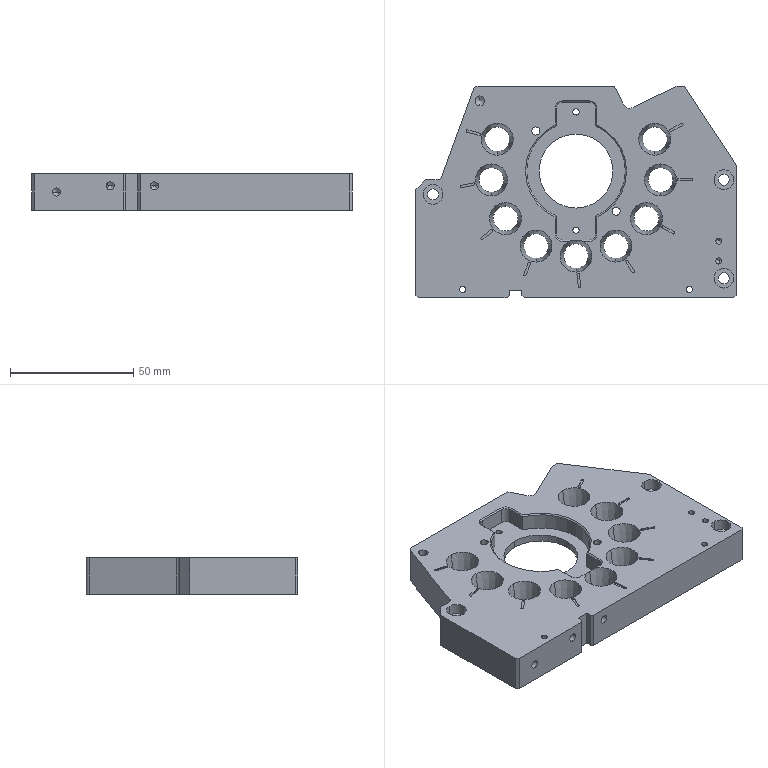NC program | NX | posted with a generic post | part box 130 x 86 x 15 mm
Lines 1 to 920 of 5031:
N10 G17 G21 G94 G90
(ADAPTIVE_MILLING_COPY , TOOL : D10)
N12 T04 M6
N14 G54
N16 G17 G0 G90 X11.01 Y-3.735 B0. C0. S7500 M3
N18 G43 Z30. H4
N20 Z3.
N22 G94 G3 X11.01 Y-3.735 Z2.506 I-2.51 J3.735 F1000.
N24 X11.01 Y-3.735 Z2.013 I-2.51 J3.735
N26 X11.01 Y-3.735 Z1.519 I-2.51 J3.735
N28 X11.01 Y-3.735 Z1.026 I-2.51 J3.735
N30 X11.01 Y-3.735 Z0.532 I-2.51 J3.735
N32 X11.01 Y-3.735 Z0.039 I-2.51 J3.735
N34 X11.01 Y-3.735 Z-0.455 I-2.51 J3.735
N36 X11.01 Y-3.735 Z-0.948 I-2.51 J3.735
N38 X11.01 Y-3.735 Z-1.442 I-2.51 J3.735
N40 X11.01 Y-3.735 Z-1.935 I-2.51 J3.735
N42 X11.01 Y-3.735 Z-2.429 I-2.51 J3.735
N44 X11.01 Y-3.735 Z-2.922 I-2.51 J3.735
N46 X11.01 Y-3.735 Z-3.416 I-2.51 J3.735
N48 X11.01 Y-3.735 Z-3.909 I-2.51 J3.735
N50 X11.01 Y-3.735 Z-4.403 I-2.51 J3.735
N52 X8.5 Y-4.5 Z-4.85 R-4.5
N54 X7.534 Y-4.399 R-4.499 F3000.
N56 X7.216 Y4.39 R-4.547
N58 X13.113 Y0.575 R-4.602
N60 X8.819 Y-4.663 R-4.652
N62 X4.804 Y2.943 R-4.71
N64 X10.9 Y4.161 R-4.762
N66 X10.384 Y-4.465 R-4.814
N68 X3.834 Y-1.432 R-4.875
N70 X7.652 Y4.886 R-4.926
N72 X13.531 Y-0.204 R-4.986
N74 X8.679 Y-5.061 R-5.039
N76 X4.13 Y2.665 R-5.102
N78 X10.535 Y4.785 R-5.156
N80 X11.506 Y-4.309 R-5.215
N82 X4.9 Y-3.869 R-5.277
N84 X6.445 Y4.953 R-5.333
N86 X13.444 Y2.278 R-5.398
N88 X9.278 Y-5.426 R-5.452
N90 X3.211 Y1.618 R-5.516
N92 X9.379 Y5.545 R-5.571
N94 X12.858 Y-3.644 R-5.637
N96 X5.804 Y-5.037 R-5.698
N98 X5.483 Y4.937 R-5.759
N100 X13.196 Y3.521 R-5.825
N102 X9.953 Y-5.735 R-5.882
N104 X2.549 Y0.352 R-5.949
N106 X9.096 Y6.019 R-6.007
N108 X13.682 Y-3.259 R-6.074
N110 X5.984 Y-5.618 R-6.137
N112 X5.083 Y5.205 R-6.201
N114 X13.852 Y3.35 R-6.267
N116 X9.625 Y-6.261 R-6.327
N118 X2.135 Y0.757 R-6.396
N120 X9.87 Y6.355 R-6.457
N122 X13.697 Y-4.024 R-6.526
N124 X4.883 Y-5.533 R-6.591
N126 X5.308 Y5.875 R-6.658
N128 X14.682 Y2.776 R-6.726
N130 X9.232 Y-6.786 R-6.79
N132 X1.734 Y1.224 R-6.86
N134 X10.363 Y6.717 R-6.925
N136 X14.11 Y-4.259 R-6.996
N138 X4.048 Y-5.51 R-7.064
N140 X5.623 Y6.56 R-7.132
N142 X15.557 Y1.686 R-7.203
N144 X8.369 Y-7.302 R-7.269
N146 X1.72 Y2.864 R-7.341
N148 X11.996 Y6.587 R-7.409
N150 X13.441 Y-5.676 R-7.48
N152 X2.184 Y-4.172 R-7.552
N154 X6.418 Y7.367 R-7.621
N156 X16.249 Y0.004 R-7.694
N158 X6.999 Y-7.65 R-7.764
N160 X1.855 Y4.197 R-7.838
N162 X13.622 Y6.092 R-7.909
N164 X12.463 Y-6.977 R-7.981
N166 X0.759 Y-2.294 R-8.055
N168 X8.58 Y8.165 R-8.126
N170 X16.024 Y-3.391 R-8.2
N172 X4.076 Y-7.019 R-8.271
N174 X3.755 Y6.902 R-8.346
N176 X16.386 Y3.104 R-8.42
N178 X9.181 Y-8.502 R-8.493
N180 X0.384 Y2.814 R-8.568
N182 X12.846 Y7.523 R-8.641
N184 X13.786 Y-6.989 R-8.716
N186 X0.145 Y-2.797 R-8.791
N188 X8.261 Y8.9 R-8.865
N190 X16.689 Y-3.723 R-8.94
N192 X2.926 Y-7.118 R-9.016
N194 X3.694 Y7.755 R-9.091
N196 X17.471 Y2.139 R-9.168
N198 X7.96 Y-9.265 R-9.244
N200 X-0.042 Y3.787 R-9.32
N202 X14.255 Y7.492 R-9.399
N204 X14. Y-7.775 R-9.475
N206 X-0.954 Y-1.506 R-9.553
N208 X10.23 Y9.516 R-9.629
N210 X16.905 Y-4.958 R-9.706
N212 X0.52 Y-5.707 R-9.784
N214 X5.806 Y9.521 R-9.861
N216 X18.258 Y-2.168 R-9.939
N218 X3.239 Y-8.561 R-10.016
N220 X2.227 Y7.946 R-10.094
N222 X18.392 Y2.605 R-10.173
N224 X8.118 Y-10.287 R-10.253
N226 X-0.877 Y4.4 R-10.332
N228 X15.771 Y7.521 R-10.413
N230 X13.155 Y-9.458 R-10.492
N232 X-2.06 Y0.845 R-10.571
N234 X12.822 Y9.783 R-10.651
N236 X16.267 Y-7.48 R-10.73
N238 X-1.831 Y-3.275 R-10.812
N240 X8.884 Y10.921 R-10.89
N242 X18.073 Y-5.475 R-10.971
N244 X-0.415 Y-6.584 R-11.051
N246 X4.875 Y10.558 R-11.132
N248 X19.445 Y-2.701 R-11.213
N250 X2.721 Y-9.748 R-11.295
N252 X1.679 Y9.143 R-11.376
N254 X19.807 Y2.176 R-11.46
N256 X7.244 Y-11.519 R-11.542
N258 X-0.899 Y6.883 R-11.623
N260 X18.674 Y5.893 R-11.706
N262 X11.097 Y-11.55 R-11.788
N264 X-2.517 Y4.491 R-11.871
N266 X16.44 Y8.998 R-11.954
N268 X13.838 Y-10.849 R-12.037
N270 X-3.507 Y1.841 R-12.119
N272 X14.292 Y10.787 R-12.202
N274 X15.907 Y-9.872 R-12.284
N276 X-3.821 Y-1.403 R-12.369
N278 X10.875 Y12.262 R-12.452
N280 X18.058 Y-8.202 R-12.537
N282 X-2.904 Y-5.494 R-12.622
N284 X7.733 Y12.715 R-12.705
N286 X19.26 Y-7.025 R-12.79
N288 X-1.417 Y-8.272 R-12.875
N290 X4.621 Y12.399 R-12.959
N292 X20.867 Y-4.326 R-13.045
N294 X0.656 Y-10.584 R-13.13
N296 X2.615 Y11.865 R-13.214
N298 X21.723 Y-1.882 R-13.301
N300 X2.704 Y-12.118 R-13.385
N302 X1.622 Y11.617 R-13.471
N304 X22.108 Y0.122 R-13.556
N306 X3.966 Y-12.919 R-13.642
N308 X1.115 Y11.607 R-13.727
N310 X22.2 Y2.124 R-13.814
N312 X5.792 Y-13.687 R-13.899
N314 X-0.216 Y10.974 R-13.986
N316 X22.159 Y3.581 R-14.072
N318 X6.615 Y-14.086 R-14.158
N320 X-0.665 Y10.944 R-14.244
N322 X22.156 Y4.493 R-14.331
N324 X6.903 Y-14.384 R-14.417
N326 X-0.683 Y11.265 R-14.504
N328 X22.47 Y4.368 R-14.59
N330 X6.639 Y-14.614 R-14.677
N332 X-0.687 Y11.599 R-14.764
N334 X22.784 Y4.222 R-14.852
N336 X5.817 Y-14.752 R-14.938
N338 X-0.232 Y12.265 R-15.026
N340 X23.361 Y2.993 R-15.113
N342 X4.981 Y-14.844 R-15.2
N344 X0.258 Y12.915 R-15.288
N346 X23.754 Y2.261 R-15.377
N348 X4.137 Y-14.894 R-15.463
N350 X1.273 Y13.806 R-15.552
N352 X24.158 Y0.954 R-15.64
N354 X2.766 Y-14.705 R-15.728
N356 X2.355 Y14.609 R-15.816
N358 X24.447 Y-0.379 R-15.905
N360 X1.423 Y-14.406 R-15.993
N362 X3.492 Y15.316 R-16.083
N364 X24.557 Y-2.283 R-16.171
N366 X0.121 Y-14. R-16.26
N368 X23.587 Y-6.301 R16.319
N370 X7.298 Y16.333 R16.374
N372 X-7.85 Y1.664 R16.374
N374 X-7.715 Y-2.654 R30.055
N376 X6.448 Y-16.35 R16.43
N378 X11.019 Y-16.271 R45.472
N380 X24.849 Y-2.38 R16.457
N382 G1 X24.85 Y0.425
N384 G3 X22.67 Y8.512 R14.212
N386 X10.995 Y16.35 R16.548
N388 X9.932 Y15.532 R1.108
N390 X10.262 Y14.424 Z-4.789 R1.127
N392 G1 X10.8 Y13.853 Z-4.75
N394 X22.33 Y1.627
N396 X22.7 Y1.23 Z-4.777
N398 X23.086 Y0.848 Z-4.804
N400 G3 X23.95 Y0.643 Z-4.85 R1.127
N402 X24.85 Y1.725 R1.106
N404 X23.606 Y7.078 R11.456
N406 X11.828 Y16.35 R16.66
N408 X10.766 Y15.535 R1.108
N410 X11.093 Y14.426 Z-4.789 R1.127
N412 G1 X11.63 Y13.853 Z-4.75
N414 X22.33 Y2.431
N416 X22.699 Y2.033 Z-4.777
N418 X23.083 Y1.65 Z-4.804
N420 G3 X23.947 Y1.442 Z-4.85 R1.127
N422 X24.85 Y2.525 R1.106
N424 X23.791 Y7.034 R9.912
N426 X12.504 Y16.349 R16.748
N428 X11.442 Y15.538 R1.108
N430 X11.765 Y14.428 Z-4.789 R1.127
N432 G1 X12.299 Y13.853 Z-4.75
N434 X22.331 Y3.061
N436 X23.059 Y2.294 Z-4.803
N438 G3 X23.943 Y2.067 Z-4.85 R1.118
N440 X24.85 Y3.15 R1.106
N442 X23.859 Y7.241 R8.92
N444 X13.073 Y16.349 R16.704
N446 X12.012 Y15.54 R1.108
N448 X12.332 Y14.43 Z-4.789 R1.127
N450 G1 X12.865 Y13.853 Z-4.75
N452 X22.331 Y3.615
N454 X23.057 Y2.846 Z-4.803
N456 G3 X23.941 Y2.616 Z-4.85 R1.118
N458 X24.85 Y3.7 R1.106
N460 X23.858 Y7.585 R8.289
N462 X13.612 Y16.345 R16.68
N464 G1 X13.587 Y16.348
N466 X13.562 Y16.35
N468 G3 X12.501 Y15.541 R1.108
N470 X12.82 Y14.432 Z-4.789 R1.127
N472 G1 X13.353 Y13.853 Z-4.75
N474 X22.331 Y4.116
N476 X23.056 Y3.347 Z-4.803
N478 G3 X23.94 Y3.116 Z-4.85 R1.118
N480 X24.85 Y4.2 R1.106
N482 X23.949 Y7.725 R7.576
N484 X14.121 Y16.339 R16.718
N486 G1 X14.096 Y16.342
N488 X14.071 Y16.345
N490 X14.046 Y16.348
N492 X14.021 Y16.35
N494 G3 X12.961 Y15.543 R1.108
N496 X13.277 Y14.433 Z-4.789 R1.127
N498 G1 X13.81 Y13.853 Z-4.75
N500 X22.331 Y4.569
N502 X23.054 Y3.798 Z-4.803
N504 G3 X23.938 Y3.566 Z-4.85 R1.117
N506 X24.85 Y4.65 R1.106
N508 X23.928 Y8.091 R7.237
N510 X14.575 Y16.334 R16.618
N512 G1 X14.551 Y16.338
N514 X14.526 Y16.342
N516 X14.501 Y16.345
N518 X14.476 Y16.347
N520 X14.451 Y16.349
N522 G3 X13.392 Y15.546 R1.108
N524 X13.705 Y14.435 Z-4.789 R1.127
N526 G1 X14.236 Y13.853 Z-4.75
N528 X22.331 Y4.974
N530 X23.051 Y4.2 Z-4.803
N532 G3 X23.934 Y3.965 Z-4.85 R1.117
N534 X24.85 Y5.05 R1.106
N536 X23.9 Y8.455 R6.966
N538 X15.025 Y16.323 R16.604
N540 G1 X15.001 Y16.328
N542 X14.976 Y16.333
N544 X14.952 Y16.338
N546 X14.927 Y16.341
N548 X14.902 Y16.344
N550 X14.877 Y16.347
N552 X14.853 Y16.349
N554 G3 X13.794 Y15.547 R1.108
N556 X14.104 Y14.437 Z-4.789 R1.127
N558 G1 X14.634 Y13.853 Z-4.75
N560 X22.331 Y5.376
N562 X23.049 Y4.602 Z-4.803
N564 G3 X23.932 Y4.365 Z-4.85 R1.117
N566 X24.85 Y5.45 R1.106
N568 X23.97 Y8.618 R6.515
N570 X15.447 Y16.312 R16.495
N572 G1 X15.422 Y16.318
N574 X15.398 Y16.324
N576 X15.374 Y16.33
N578 X15.349 Y16.334
N580 X15.325 Y16.338
N582 X15.3 Y16.342
N584 X15.275 Y16.345
N586 X15.25 Y16.348
N588 X15.225 Y16.349
N590 G3 X14.167 Y15.549 R1.108
N592 X14.476 Y14.438 Z-4.79 R1.127
N594 G1 X15.005 Y13.853 Z-4.75
N596 X22.331 Y5.754
N598 X23.048 Y4.978 Z-4.803
N600 G3 X23.931 Y4.74 Z-4.85 R1.117
N602 X24.85 Y5.825 R1.106
N604 X23.957 Y8.937 R6.318
N606 X15.839 Y16.302 R16.322
N608 G1 X15.816 Y16.309
N610 X15.791 Y16.316
N612 X15.767 Y16.322
N614 X15.743 Y16.328
N616 X15.718 Y16.333
N618 X15.694 Y16.337
N620 X15.669 Y16.341
N622 X15.644 Y16.344
N624 X15.619 Y16.347
N626 X15.594 Y16.349
N628 G3 X14.537 Y15.551 R1.108
N630 X14.842 Y14.44 Z-4.79 R1.127
N632 G1 X15.37 Y13.853 Z-4.75
N634 X22.331 Y6.108
N636 X23.045 Y5.33 Z-4.803
N638 G3 X23.928 Y5.089 Z-4.85 R1.117
N640 X24.85 Y6.175 R1.106
N642 X23.952 Y9.233 R6.12
N644 X16.276 Y16.272 R16.312
N646 G1 X16.205 Y16.296
N648 X16.157 Y16.311
N650 X16.133 Y16.317
N652 X16.108 Y16.323
N654 X16.084 Y16.329
N656 X16.059 Y16.334
N658 X16.035 Y16.338
N660 X16.01 Y16.342
N662 X15.985 Y16.345
N664 X15.96 Y16.347
N666 X15.935 Y16.349
N668 G3 X14.878 Y15.554 R1.108
N670 X15.181 Y14.443 Z-4.79 R1.127
N672 G1 X15.708 Y13.853 Z-4.75
N674 X22.331 Y6.437
N676 X23.042 Y5.658 Z-4.803
N678 G3 X23.925 Y5.414 Z-4.85 R1.117
N680 X24.85 Y6.5 R1.106
N682 X23.978 Y9.462 R5.87
N684 X16.661 Y16.253 R16.132
N686 G1 X16.59 Y16.278
N688 X16.519 Y16.302
N690 X16.495 Y16.309
N692 X16.471 Y16.316
N694 X16.447 Y16.322
N696 X16.422 Y16.328
N698 X16.398 Y16.333
N700 X16.373 Y16.337
N702 X16.348 Y16.341
N704 X16.324 Y16.344
N706 X16.299 Y16.347
N708 X16.274 Y16.349
N710 G3 X15.218 Y15.556 R1.108
N712 X15.517 Y14.445 Z-4.79 R1.127
N714 G1 X16.042 Y13.853 Z-4.75
N716 X22.331 Y6.766
N718 X23.04 Y5.985 Z-4.803
N720 G3 X23.922 Y5.738 Z-4.85 R1.117
N722 X24.85 Y6.825 R1.106
N724 X23.979 Y9.734 R5.708
N726 X16.995 Y16.248 R15.815
N728 G1 X16.925 Y16.273
N730 X16.854 Y16.298
N732 X16.83 Y16.305
N734 X16.806 Y16.312
N736 X16.782 Y16.319
N738 X16.757 Y16.325
N740 X16.733 Y16.33
N742 X16.708 Y16.335
N744 X16.684 Y16.339
N746 X16.659 Y16.342
N748 X16.634 Y16.345
N750 X16.609 Y16.348
N752 X16.584 Y16.35
N754 G3 X15.528 Y15.557 R1.108
N756 X15.826 Y14.447 Z-4.79 R1.127
N758 G1 X16.351 Y13.853 Z-4.75
N760 X22.331 Y7.093
N762 X23.039 Y6.311 Z-4.803
N764 G3 X23.92 Y6.063 Z-4.85 R1.117
N766 X24.85 Y7.15 R1.106
N768 X23.94 Y10.072 R5.658
N770 X17.349 Y16.23 R15.574
N772 G1 X17.28 Y16.257
N774 X17.209 Y16.283
N776 X17.162 Y16.299
N778 X17.138 Y16.306
N780 X17.114 Y16.313
N782 X17.09 Y16.319
N784 X17.065 Y16.325
N786 X17.041 Y16.33
N788 X17.016 Y16.335
N790 X16.992 Y16.339
N792 X16.967 Y16.343
N794 X16.942 Y16.346
N796 X16.917 Y16.348
N798 X16.892 Y16.35
N800 G3 X15.837 Y15.559 R1.108
N802 X16.132 Y14.449 Z-4.79 R1.128
N804 G1 X16.656 Y13.853 Z-4.75
N806 X22.331 Y7.398
N808 X23.036 Y6.613 Z-4.803
N810 G3 X23.917 Y6.363 Z-4.85 R1.117
N812 X24.85 Y7.45 R1.106
N814 X23.934 Y10.343 R5.537
N816 X17.677 Y16.219 R15.23
N818 G1 X17.608 Y16.247
N820 X17.538 Y16.273
N822 X17.467 Y16.298
N824 X17.443 Y16.305
N826 X17.419 Y16.312
N828 X17.395 Y16.319
N830 X17.37 Y16.325
N832 X17.346 Y16.33
N834 X17.321 Y16.335
N836 X17.297 Y16.339
N838 X17.272 Y16.342
N840 X17.247 Y16.345
N842 X17.222 Y16.348
N844 X17.197 Y16.35
N846 G3 X16.143 Y15.562 R1.108
N848 X16.434 Y14.451 Z-4.79 R1.128
N850 G1 X16.957 Y13.853 Z-4.75
N852 X22.331 Y7.702
N854 X23.033 Y6.915 Z-4.803
N856 G3 X23.914 Y6.662 Z-4.85 R1.117
N858 X24.85 Y7.75 R1.106
N860 X23.951 Y10.571 R5.394
N862 X17.933 Y16.234 R14.657
N864 G1 X17.863 Y16.261
N866 X17.793 Y16.287
N868 X17.745 Y16.303
N870 X17.721 Y16.31
N872 X17.697 Y16.317
N874 X17.673 Y16.323
N876 X17.648 Y16.328
N878 X17.624 Y16.333
N880 X17.599 Y16.337
N882 X17.575 Y16.341
N884 X17.55 Y16.344
N886 X17.525 Y16.347
N888 X17.5 Y16.349
N890 G3 X16.446 Y15.565 R1.108
N892 X16.733 Y14.454 Z-4.79 R1.128
N894 G1 X17.253 Y13.853 Z-4.75
N896 X22.331 Y7.983
N898 X23.029 Y7.194 Z-4.803
N900 G3 X23.909 Y6.936 Z-4.85 R1.117
N902 X24.85 Y8.025 R1.106
N904 X23.94 Y10.841 R5.294
N906 X18.255 Y16.218 R14.31
N908 G1 X18.186 Y16.247
N910 X18.116 Y16.274
N912 X18.069 Y16.29
N914 X18.045 Y16.298
N916 X18.021 Y16.306
N918 X17.997 Y16.313
N920 X17.973 Y16.319
N922 X17.949 Y16.325
N924 X17.924 Y16.33
N926 X17.9 Y16.335
N928 X17.875 Y16.339
N930 X17.85 Y16.343
N932 X17.825 Y16.346
N934 X17.801 Y16.348
N936 X17.776 Y16.35
N938 G3 X16.722 Y15.566 R1.108
N940 X17.008 Y14.456 Z-4.79 R1.128
N942 G1 X17.528 Y13.853 Z-4.75
N944 X22.331 Y8.285
N946 X23.028 Y7.495 Z-4.803
N948 G3 X23.908 Y7.236 Z-4.85 R1.117
N950 X24.85 Y8.325 R1.106
N952 X23.966 Y11.046 R5.156
N954 X18.552 Y16.21 R13.864
N956 G1 X18.049 Y16.35
N958 G3 X16.996 Y15.568 R1.108
N960 X17.279 Y14.458 Z-4.79 R1.128
N962 G1 X17.798 Y13.853 Z-4.75
N964 X22.332 Y8.564
N966 X23.026 Y7.772 Z-4.803
N968 G3 X23.905 Y7.511 Z-4.85 R1.117
N970 X24.85 Y8.6 R1.106
N972 X23.912 Y11.38 R5.187
N974 X18.845 Y16.201 R13.419
N976 G1 X18.777 Y16.23
N978 X18.707 Y16.259
N980 X18.637 Y16.285
N982 X18.589 Y16.301
N984 X18.566 Y16.308
N986 X18.542 Y16.315
N988 X18.517 Y16.321
N990 X18.493 Y16.327
N992 X18.468 Y16.332
N994 X18.444 Y16.336
N996 X18.419 Y16.34
N998 X18.394 Y16.344
N1000 X18.37 Y16.346
N1002 X18.345 Y16.349
N1004 G3 X17.294 Y15.574 R1.108
N1006 X17.569 Y14.463 Z-4.79 R1.128
N1008 G1 X18.084 Y13.853 Z-4.75
N1010 X22.332 Y8.824
N1012 X23.02 Y8.027 Z-4.803
N1014 G3 X23.898 Y7.76 Z-4.85 R1.117
N1016 X24.85 Y8.85 R1.106
N1018 X23.986 Y11.498 R4.938
N1020 X19.091 Y16.209 R12.81
N1022 G1 X19.022 Y16.239
N1024 X18.975 Y16.258
N1026 X18.905 Y16.284
N1028 X18.858 Y16.3
N1030 X18.834 Y16.308
N1032 X18.81 Y16.315
N1034 X18.786 Y16.321
N1036 X18.762 Y16.327
N1038 X18.737 Y16.332
N1040 X18.713 Y16.336
N1042 X18.688 Y16.34
N1044 X18.663 Y16.343
N1046 X18.638 Y16.346
N1048 X18.613 Y16.348
N1050 G3 X17.563 Y15.577 R1.108
N1052 X17.835 Y14.465 Z-4.79 R1.128
N1054 G1 X18.348 Y13.853 Z-4.75
N1056 X22.332 Y9.104
N1058 X23.017 Y8.305 Z-4.803
N1060 G3 X23.894 Y8.034 Z-4.85 R1.117
N1062 X24.85 Y9.125 R1.106
N1064 X23.929 Y11.831 R4.984
N1066 X19.356 Y16.206 R12.272
N1068 G1 X18.855 Y16.35
N1070 G3 X17.805 Y15.579 R1.108
N1072 X18.125 Y14.407 Z-4.786 R1.183
N1074 G1 X18.587 Y13.853 Z-4.75
N1076 X22.332 Y9.358
N1078 X23.014 Y8.557 Z-4.803
N1080 G3 X23.891 Y8.284 Z-4.85 R1.117
N1082 X24.85 Y9.375 R1.106
N1084 X23.922 Y12.078 R4.925
N1086 X19.574 Y16.222 R11.593
N1088 G1 X19.528 Y16.242
N1090 X19.458 Y16.27
N1092 X19.411 Y16.287
N1094 X19.388 Y16.295
N1096 X19.364 Y16.303
N1098 X19.34 Y16.31
N1100 X19.316 Y16.317
N1102 X19.292 Y16.323
N1104 X19.267 Y16.328
N1106 X19.243 Y16.333
N1108 X19.218 Y16.338
N1110 X19.194 Y16.341
N1112 X19.169 Y16.344
N1114 X19.144 Y16.347
N1116 X19.119 Y16.349
N1118 G3 X18.071 Y15.583 R1.108
N1120 X18.385 Y14.41 Z-4.786 R1.183
N1122 G1 X18.844 Y13.853 Z-4.75
N1124 X22.332 Y9.616
N1126 X23.01 Y8.811 Z-4.803
N1128 G3 X23.885 Y8.533 Z-4.85 R1.117
N1130 X24.85 Y9.625 R1.106
N1132 X23.966 Y12.239 R4.766
N1134 X19.789 Y16.236 R10.943
N1136 G1 X19.719 Y16.265
N1138 X19.673 Y16.283
N1140 X19.649 Y16.291
N1142 X19.626 Y16.299
N1144 X19.602 Y16.307
N1146 X19.578 Y16.314
N1148 X19.554 Y16.32
N1150 X19.529 Y16.326
N1152 X19.505 Y16.331
N1154 X19.48 Y16.335
N1156 X19.456 Y16.339
N1158 X19.431 Y16.343
N1160 X19.406 Y16.346
N1162 X19.381 Y16.348
N1164 X19.356 Y16.35
N1166 G3 X18.308 Y15.584 R1.108
N1168 X18.621 Y14.412 Z-4.786 R1.184
N1170 G1 X19.08 Y13.853 Z-4.75
N1172 X22.332 Y9.893
N1174 X23.009 Y9.087 Z-4.803
N1176 G3 X23.883 Y8.808 Z-4.85 R1.117
N1178 X24.85 Y9.9 R1.106
N1180 X23.956 Y12.484 R4.742
N1182 X20.07 Y16.219 R10.506
N1184 G1 X20.001 Y16.249
N1186 X19.955 Y16.268
N1188 X19.908 Y16.285
N1190 X19.885 Y16.294
N1192 X19.861 Y16.302
N1194 X19.837 Y16.309
N1196 X19.813 Y16.316
N1198 X19.789 Y16.322
N1200 X19.764 Y16.327
N1202 X19.74 Y16.332
N1204 X19.715 Y16.337
N1206 X19.691 Y16.341
N1208 X19.666 Y16.344
N1210 X19.641 Y16.347
N1212 X19.616 Y16.349
N1214 G3 X18.76 Y14.558 R1.101
N1216 G1 X22.894 Y9.434
N1218 G3 X24.85 Y10.125 R1.101
N1220 X23.944 Y12.73 R4.686
N1222 X20.234 Y16.251 R9.703
N1224 G1 X20.188 Y16.269
N1226 X20.141 Y16.287
N1228 X20.118 Y16.295
N1230 X20.094 Y16.303
N1232 X20.07 Y16.31
N1234 X20.046 Y16.317
N1236 X20.021 Y16.323
N1238 X19.997 Y16.328
N1240 X19.973 Y16.333
N1242 X19.948 Y16.338
N1244 X19.923 Y16.341
N1246 X19.898 Y16.345
N1248 X19.874 Y16.347
N1250 X19.849 Y16.349
N1252 G3 X18.99 Y14.562 R1.101
N1254 G1 X22.891 Y9.687
N1256 G3 X24.85 Y10.375 R1.101
N1258 X23.957 Y12.932 R4.601
N1260 X20.488 Y16.241 R9.232
N1262 G1 X20.418 Y16.27
N1264 X20.372 Y16.288
N1266 X20.348 Y16.296
N1268 X20.324 Y16.304
N1270 X20.3 Y16.311
N1272 X20.276 Y16.318
N1274 X20.252 Y16.323
N1276 X20.227 Y16.329
N1278 X20.203 Y16.334
N1280 X20.178 Y16.338
N1282 X20.154 Y16.342
N1284 X20.129 Y16.345
N1286 X20.104 Y16.347
N1288 X20.079 Y16.349
N1290 G3 X19.217 Y14.565 R1.101
N1292 G1 X22.888 Y9.941
N1294 G3 X24.85 Y10.625 R1.101
N1296 X23.956 Y13.155 R4.556
N1298 X20.646 Y16.27 R8.483
N1300 G1 X20.6 Y16.287
N1302 X20.576 Y16.296
N1304 X20.552 Y16.304
N1306 X20.528 Y16.311
N1308 X20.504 Y16.317
N1310 X20.48 Y16.323
N1312 X20.455 Y16.329
N1314 X20.431 Y16.334
N1316 X20.406 Y16.338
N1318 X20.382 Y16.341
N1320 X20.357 Y16.345
N1322 X20.332 Y16.347
N1324 X20.307 Y16.349
N1326 G3 X19.441 Y14.571 R1.101
N1328 G1 X22.884 Y10.172
N1330 G3 X24.85 Y10.85 R1.101
N1332 X23.952 Y13.378 R4.485
N1334 X20.825 Y16.286 R7.814
N1336 G1 X20.801 Y16.294
N1338 X20.777 Y16.302
N1340 X20.754 Y16.309
N1342 X20.729 Y16.316
N1344 X20.705 Y16.322
N1346 X20.681 Y16.328
N1348 X20.656 Y16.333
N1350 X20.632 Y16.337
N1352 X20.607 Y16.341
N1354 X20.582 Y16.344
N1356 X20.557 Y16.347
N1358 X20.532 Y16.349
N1360 G3 X19.663 Y14.575 R1.101
N1362 G1 X22.881 Y10.426
N1364 G3 X24.85 Y11.1 R1.101
N1366 X23.919 Y13.641 R4.482
N1368 X21. Y16.3 R7.136
N1370 G1 X20.976 Y16.307
N1372 X20.952 Y16.314
N1374 X20.928 Y16.32
N1376 X20.903 Y16.326
N1378 X20.879 Y16.331
N1380 X20.854 Y16.336
N1382 X20.83 Y16.34
N1384 X20.805 Y16.343
N1386 X20.78 Y16.346
N1388 X20.755 Y16.348
N1390 X20.73 Y16.35
N1392 G3 X19.858 Y14.579 R1.101
N1394 G1 X22.878 Y10.654
N1396 G3 X24.85 Y11.325 R1.101
N1398 X23.924 Y13.841 R4.392
N1400 X21.196 Y16.304 R6.608
N1402 G1 X21.172 Y16.311
N1404 X21.148 Y16.318
N1406 X21.123 Y16.324
N1408 X21.099 Y16.329
N1410 X21.074 Y16.334
N1412 X21.05 Y16.338
N1414 X21.025 Y16.342
N1416 X21. Y16.345
N1418 X20.975 Y16.347
N1420 X20.951 Y16.349
N1422 G3 X20.073 Y14.586 R1.101
N1424 G1 X22.873 Y10.886
N1426 G3 X24.85 Y11.55 R1.101
N1428 X23.914 Y14.06 R4.328
N1430 X21.365 Y16.314 R5.974
N1432 G1 X21.34 Y16.32
N1434 X21.316 Y16.326
N1436 X21.292 Y16.331
N1438 X21.267 Y16.336
N1440 X21.242 Y16.34
N1442 X21.218 Y16.343
N1444 X21.193 Y16.346
N1446 X21.168 Y16.348
N1448 X21.143 Y16.35
N1450 G3 X20.263 Y14.59 R1.101
N1452 G1 X22.87 Y11.115
N1454 G3 X24.85 Y11.775 R1.101
N1456 X23.9 Y14.279 R4.253
N1458 X21.555 Y16.316 R5.484
N1460 G1 X21.53 Y16.322
N1462 X21.506 Y16.328
N1464 X21.481 Y16.333
N1466 X21.457 Y16.337
N1468 X21.432 Y16.341
N1470 X21.407 Y16.344
N1472 X21.382 Y16.347
N1474 X21.358 Y16.349
N1476 G3 X20.472 Y14.597 R1.101
N1478 G1 X22.864 Y11.347
N1480 G3 X24.85 Y12. R1.101
N1482 X23.837 Y14.555 R4.235
N1484 X21.693 Y16.328 R4.734
N1486 G1 X21.668 Y16.333
N1488 X21.643 Y16.338
N1490 X21.619 Y16.341
N1492 X21.594 Y16.345
N1494 X21.569 Y16.347
N1496 X21.544 Y16.349
N1498 G3 X20.655 Y14.601 R1.101
N1500 G1 X22.861 Y11.577
N1502 G3 X24.85 Y12.225 R1.101
N1504 X23.799 Y14.789 R4.168
N1506 X21.852 Y16.334 R4.158
N1508 G1 X21.827 Y16.338
N1510 X21.802 Y16.342
N1512 X21.777 Y16.345
N1514 X21.753 Y16.347
N1516 X21.728 Y16.349
N1518 G3 X20.833 Y14.609 R1.101
N1520 G1 X22.856 Y11.784
N1522 G3 X24.85 Y12.425 R1.101
N1524 X23.833 Y14.921 R3.992
N1526 X22.007 Y16.337 R3.732
N1528 G1 X21.982 Y16.341
N1530 X21.958 Y16.344
N1532 X21.933 Y16.347
N1534 X21.908 Y16.349
N1536 G3 X21.01 Y14.613 R1.101
N1538 G1 X22.853 Y12.014
N1540 G3 X24.85 Y12.65 R1.101
N1542 X23.736 Y15.206 R3.957
N1544 X22.134 Y16.344 R3.07
N1546 G1 X22.11 Y16.347
N1548 X22.085 Y16.349
N1550 G3 X21.181 Y14.621 R1.101
N1552 G1 X22.846 Y12.222
N1554 G3 X24.85 Y12.85 R1.101
N1556 X23.677 Y15.427 R3.841
N1558 X22.233 Y16.35 R2.494
N1560 X21.327 Y14.625 R1.101
N1562 G1 X22.844 Y12.425
N1564 G3 X24.85 Y13.05 R1.101
N1566 X23.625 Y15.623 R3.697
N1568 X22.403 Y16.349 R2.184
N1570 X21.49 Y14.634 R1.101
N1572 G1 X22.838 Y12.635
N1574 G3 X24.85 Y13.25 R1.101
N1576 X22.717 Y16.325 R3.526
N1578 G1 X22.692 Y16.33
N1580 X22.668 Y16.335
N1582 X22.643 Y16.339
N1584 X22.618 Y16.342
N1586 X22.594 Y16.345
N1588 X22.569 Y16.348
N1590 X22.544 Y16.35
N1592 G3 X21.63 Y14.637 R1.102
N1594 G1 X22.836 Y12.837
N1596 G3 X24.85 Y13.45 R1.101
N1598 X22.854 Y16.326 R3.256
N1600 G1 X22.83 Y16.331
N1602 X22.805 Y16.336
N1604 X22.78 Y16.34
N1606 X22.756 Y16.343
N1608 X22.731 Y16.346
N1610 X22.706 Y16.348
N1612 X22.681 Y16.35
N1614 G3 X21.762 Y14.645 R1.102
N1616 G1 X22.831 Y13.02
N1618 G3 X24.85 Y13.625 R1.101
N1620 X22.987 Y16.327 R3.004
N1622 G1 X22.963 Y16.332
N1624 X22.938 Y16.336
N1626 X22.914 Y16.34
N1628 X22.889 Y16.344
N1630 X22.864 Y16.346
N1632 X22.839 Y16.349
N1634 G3 X21.908 Y14.663 R1.102
N1636 G1 X22.819 Y13.214
N1638 G3 X24.85 Y13.8 R1.101
N1640 X23.117 Y16.327 R2.772
N1642 G1 X23.092 Y16.332
N1644 X23.067 Y16.337
N1646 X23.043 Y16.34
N1648 X23.018 Y16.344
N1650 X22.993 Y16.346
N1652 X22.968 Y16.349
N1654 G3 X22.031 Y14.673 R1.102
N1656 G1 X22.812 Y13.399
N1658 G3 X24.85 Y13.975 R1.101
N1660 X23.217 Y16.332 R2.522
N1662 G1 X23.192 Y16.336
N1664 X23.168 Y16.34
N1666 X23.143 Y16.343
N1668 X23.118 Y16.346
N1670 X23.093 Y16.348
N1672 X23.068 Y16.35
N1674 G3 X22.133 Y14.671 R1.102
N1676 G1 X22.516 Y14.042
N1678 X22.92 Y13.427
N1680 G3 X24.85 Y14.15 R1.101
N1682 X23.313 Y16.335 R2.298
N1684 G1 X23.289 Y16.339
N1686 X23.264 Y16.343
N1688 X23.239 Y16.346
N1690 X23.214 Y16.348
N1692 X23.189 Y16.35
N1694 G3 X22.242 Y14.691 R1.102
N1696 G1 X22.564 Y14.136
N1698 X22.906 Y13.594
N1700 G3 X24.85 Y14.3 R1.101
N1702 X23.405 Y16.338 R2.096
N1704 G1 X23.38 Y16.341
N1706 X23.356 Y16.344
N1708 X23.331 Y16.347
N1710 X23.306 Y16.349
N1712 G3 X22.344 Y14.715 R1.102
N1714 G1 X22.607 Y14.234
N1716 X22.889 Y13.765
N1718 G3 X24.85 Y14.45 R1.101
N1720 X23.493 Y16.339 R1.914
N1722 G1 X23.468 Y16.343
N1724 X23.443 Y16.346
N1726 X23.418 Y16.348
N1728 X23.393 Y16.35
N1730 G3 X22.429 Y14.721 R1.102
N1732 G1 X22.649 Y14.315
N1734 X22.886 Y13.919
N1736 G3 X24.85 Y14.6 R1.101
N1738 X23.526 Y16.347 R1.719
N1740 G1 X23.501 Y16.349
N1742 G3 X22.517 Y14.758 R1.102
N1744 G1 X22.855 Y14.111
N1746 G3 X24.85 Y14.75 R1.101
N1748 X23.581 Y16.349 R1.562
N1750 X22.578 Y14.796 R1.102
N1752 G1 X22.833 Y14.268
N1754 G3 X24.85 Y14.875 R1.101
N1756 X23.656 Y16.349 R1.433
N1758 X23.31 Y13.793 R1.301
N1760 X24.85 Y15. R1.246
N1762 X23.726 Y16.349 R1.317
N1764 X22.726 Y14.617 R1.499
N1766 G1 Z-1.85
N1768 G0 Z30.
N1770 X22.918 Y14.582
N1772 Z-1.85
N1774 G1 Z-4.85 F1000.
N1776 G3 X24.85 Y15.1 R1.051 F3000.
N1778 X23.717 Y16.35 R1.2
N1780 G1 X9.667
N1782 G3 X8.569 Y15.248 R1.1
N1784 X9.663 Y14.15 R1.1
N1786 G1 X23.746 Y14.1
N1788 G3 X24.844 Y15.303 R1.103
N1790 X24.526 Y16.022 R1.306
N1792 X24.43 Y14.642 R-0.923
N1794 X24.749 Y15.692 R0.939
N1796 X24.002 Y16.309 R1.061
N1798 G1 X23.717 Y16.35
N1800 X7.822
N1802 G3 X0.412 Y14.452 R13.751
N1804 X-7.849 Y2.767 R16.544
N1806 X-7.037 Y1.706 R1.108
N1808 X-5.927 Y2.029 Z-4.789 R1.127
N1810 G1 X-5.353 Y2.564 Z-4.75
N1812 X6.738 Y13.83
N1814 X7.137 Y14.198 Z-4.777
N1816 X7.52 Y14.581 Z-4.804
N1818 G3 X7.73 Y15.444 Z-4.85 R1.127
N1820 X6.647 Y16.35 R1.106
N1822 X1.505 Y15.176 R11.153
N1824 X-7.85 Y3.523 R16.644
N1826 X-7.038 Y2.462 R1.108
N1828 X-5.929 Y2.784 Z-4.789 R1.127
N1830 G1 X-5.353 Y3.32 Z-4.75
N1832 X5.961 Y13.831
N1834 X6.728 Y14.559 Z-4.803
N1836 G3 X6.955 Y15.443 Z-4.85 R1.118
N1838 X5.872 Y16.35 R1.106